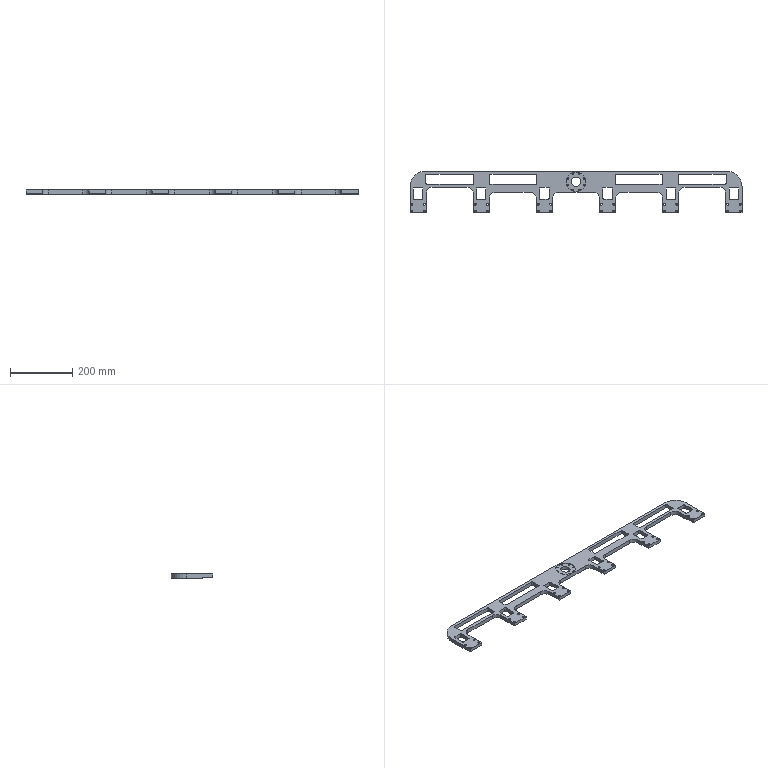NC program | NX | posted with a generic post | part box 1068 x 134 x 13 mm
Lines 5044 to 6064 of 9724:
(HOLE_MILLING_COPY , TOOL : D6)
N10038 T06 M6
N10040 G54
N10042 G17 G0 G90 X-25.869 Y43.715 S9500 M3
N10044 G43 Z30. H6
N10046 Z0.5
N10048 G94 G3 X-26.369 Y44.215 R0.5 F1400.
N10050 X-26.869 Y43.715 R0.5
N10052 X-26.869 Y43.715 Z0. I1. J0.
N10054 X-26.869 Y43.715 Z-0.5 I1. J0.
N10056 X-26.869 Y43.715 Z-1. I1. J0.
N10058 X-26.869 Y43.715 Z-1.5 I1. J0.
N10060 X-26.869 Y43.715 Z-2. I1. J0.
N10062 X-26.869 Y43.715 Z-2.5 I1. J0.
N10064 X-26.869 Y43.715 Z-3. I1. J0.
N10066 X-26.869 Y43.715 Z-3.5 I1. J0.
N10068 X-26.869 Y43.715 Z-4. I1. J0.
N10070 X-26.869 Y43.715 Z-4.5 I1. J0.
N10072 X-26.178 Y42.764 Z-4.6 R1.
N10074 X-24.918 Y43.406 R1.
N10076 X-26.178 Y42.764 R-1.
N10078 X-25.548 Y43.085 R0.5
N10080 X-25.869 Y43.715 R0.5
N10082 G0 Z30.
N10084 Y22.285
N10086 Z0.5
N10088 G3 X-26.369 Y22.785 R0.5
N10090 X-26.869 Y22.285 R0.5
N10092 X-26.869 Y22.285 Z0. I1. J0.
N10094 X-26.869 Y22.285 Z-0.5 I1. J0.
N10096 X-26.869 Y22.285 Z-1. I1. J0.
N10098 X-26.869 Y22.285 Z-1.5 I1. J0.
N10100 X-26.869 Y22.285 Z-2. I1. J0.
N10102 X-26.869 Y22.285 Z-2.5 I1. J0.
N10104 X-26.869 Y22.285 Z-3. I1. J0.
N10106 X-26.869 Y22.285 Z-3.5 I1. J0.
N10108 X-26.869 Y22.285 Z-4. I1. J0.
N10110 X-26.869 Y22.285 Z-4.5 I1. J0.
N10112 X-26.178 Y21.334 Z-4.6 R1.
N10114 X-24.918 Y21.976 R1.
N10116 X-26.178 Y21.334 R-1.
N10118 X-25.548 Y21.655 R0.5
N10120 X-25.869 Y22.285 R0.5
N10122 G0 Z30.
N10124 X-10.715 Y7.131
N10126 Z0.5
N10128 G3 X-11.215 Y7.631 R0.5
N10130 X-11.715 Y7.131 R0.5
N10132 X-11.715 Y7.131 Z0. I1. J0.
N10134 X-11.715 Y7.131 Z-0.5 I1. J0.
N10136 X-11.715 Y7.131 Z-1. I1. J0.
N10138 X-11.715 Y7.131 Z-1.5 I1. J0.
N10140 X-11.715 Y7.131 Z-2. I1. J0.
N10142 X-11.715 Y7.131 Z-2.5 I1. J0.
N10144 X-11.715 Y7.131 Z-3. I1. J0.
N10146 X-11.715 Y7.131 Z-3.5 I1. J0.
N10148 X-11.715 Y7.131 Z-4. I1. J0.
N10150 X-11.715 Y7.131 Z-4.5 I1. J0.
N10152 X-11.024 Y6.18 Z-4.6 R1.
N10154 X-9.764 Y6.822 R1.
N10156 X-11.024 Y6.18 R-1.
N10158 X-10.394 Y6.501 R0.5
N10160 X-10.715 Y7.131 R0.5
N10162 G0 Z30.
N10164 X10.715
N10166 Z0.5
N10168 G3 X10.215 Y7.631 R0.5
N10170 X9.715 Y7.131 R0.5
N10172 X9.715 Y7.131 Z0. I1. J0.
N10174 X9.715 Y7.131 Z-0.5 I1. J0.
N10176 X9.715 Y7.131 Z-1. I1. J0.
N10178 X9.715 Y7.131 Z-1.5 I1. J0.
N10180 X9.715 Y7.131 Z-2. I1. J0.
N10182 X9.715 Y7.131 Z-2.5 I1. J0.
N10184 X9.715 Y7.131 Z-3. I1. J0.
N10186 X9.715 Y7.131 Z-3.5 I1. J0.
N10188 X9.715 Y7.131 Z-4. I1. J0.
N10190 X9.715 Y7.131 Z-4.5 I1. J0.
N10192 X10.406 Y6.18 Z-4.6 R1.
N10194 X11.666 Y6.822 R1.
N10196 X10.406 Y6.18 R-1.
N10198 X11.036 Y6.501 R0.5
N10200 X10.715 Y7.131 R0.5
N10202 G0 Z30.
N10204 X25.869 Y22.285
N10206 Z0.5
N10208 G3 X25.369 Y22.785 R0.5
N10210 X24.869 Y22.285 R0.5
N10212 X24.869 Y22.285 Z0. I1. J0.
N10214 X24.869 Y22.285 Z-0.5 I1. J0.
N10216 X24.869 Y22.285 Z-1. I1. J0.
N10218 X24.869 Y22.285 Z-1.5 I1. J0.
N10220 X24.869 Y22.285 Z-2. I1. J0.
N10222 X24.869 Y22.285 Z-2.5 I1. J0.
N10224 X24.869 Y22.285 Z-3. I1. J0.
N10226 X24.869 Y22.285 Z-3.5 I1. J0.
N10228 X24.869 Y22.285 Z-4. I1. J0.
N10230 X24.869 Y22.285 Z-4.5 I1. J0.
N10232 X25.56 Y21.334 Z-4.6 R1.
N10234 X26.82 Y21.976 R1.
N10236 X25.56 Y21.334 R-1.
N10238 X26.19 Y21.655 R0.5
N10240 X25.869 Y22.285 R0.5
N10242 G0 Z30.
N10244 Y43.715
N10246 Z0.5
N10248 G3 X25.369 Y44.215 R0.5
N10250 X24.869 Y43.715 R0.5
N10252 X24.869 Y43.715 Z0. I1. J0.
N10254 X24.869 Y43.715 Z-0.5 I1. J0.
N10256 X24.869 Y43.715 Z-1. I1. J0.
N10258 X24.869 Y43.715 Z-1.5 I1. J0.
N10260 X24.869 Y43.715 Z-2. I1. J0.
N10262 X24.869 Y43.715 Z-2.5 I1. J0.
N10264 X24.869 Y43.715 Z-3. I1. J0.
N10266 X24.869 Y43.715 Z-3.5 I1. J0.
N10268 X24.869 Y43.715 Z-4. I1. J0.
N10270 X24.869 Y43.715 Z-4.5 I1. J0.
N10272 X25.56 Y42.764 Z-4.6 R1.
N10274 X26.82 Y43.406 R1.
N10276 X25.56 Y42.764 R-1.
N10278 X26.19 Y43.085 R0.5
N10280 X25.869 Y43.715 R0.5
N10282 G0 Z30.
N10284 X10.715 Y58.869
N10286 Z0.5
N10288 G3 X10.215 Y59.369 R0.5
N10290 X9.715 Y58.869 R0.5
N10292 X9.715 Y58.869 Z0. I1. J0.
N10294 X9.715 Y58.869 Z-0.5 I1. J0.
N10296 X9.715 Y58.869 Z-1. I1. J0.
N10298 X9.715 Y58.869 Z-1.5 I1. J0.
N10300 X9.715 Y58.869 Z-2. I1. J0.
N10302 X9.715 Y58.869 Z-2.5 I1. J0.
N10304 X9.715 Y58.869 Z-3. I1. J0.
N10306 X9.715 Y58.869 Z-3.5 I1. J0.
N10308 X9.715 Y58.869 Z-4. I1. J0.
N10310 X9.715 Y58.869 Z-4.5 I1. J0.
N10312 X10.406 Y57.918 Z-4.6 R1.
N10314 X11.666 Y58.56 R1.
N10316 X10.406 Y57.918 R-1.
N10318 X11.036 Y58.239 R0.5
N10320 X10.715 Y58.869 R0.5
N10322 G0 Z30.
N10324 X-10.715
N10326 Z0.5
N10328 G3 X-11.215 Y59.369 R0.5
N10330 X-11.715 Y58.869 R0.5
N10332 X-11.715 Y58.869 Z0. I1. J0.
N10334 X-11.715 Y58.869 Z-0.5 I1. J0.
N10336 X-11.715 Y58.869 Z-1. I1. J0.
N10338 X-11.715 Y58.869 Z-1.5 I1. J0.
N10340 X-11.715 Y58.869 Z-2. I1. J0.
N10342 X-11.715 Y58.869 Z-2.5 I1. J0.
N10344 X-11.715 Y58.869 Z-3. I1. J0.
N10346 X-11.715 Y58.869 Z-3.5 I1. J0.
N10348 X-11.715 Y58.869 Z-4. I1. J0.
N10350 X-11.715 Y58.869 Z-4.5 I1. J0.
N10352 X-11.024 Y57.918 Z-4.6 R1.
N10354 X-9.764 Y58.56 R1.
N10356 X-11.024 Y57.918 R-1.
N10358 X-10.394 Y58.239 R0.5
N10360 X-10.715 Y58.869 R0.5
N10362 G0 Z30.
(ZLEVEL_PROFILE_COPY_1_COPY , TOOL : D6)
N10364 X-131.879 Y29.2
N10366 Z-0.591
N10368 G1 Y28.003 F1000.
N10370 X-131.816 Y28.
N10372 X-129.6 F1650.
N10374 Y30.216
N10376 X-129.603 Y30.279
N10378 X-130.8
N10380 G0 X-131.879 Y29.2 Z-1.182
N10382 G1 Y28.003 F1000.
N10384 X-131.816 Y28.
N10386 X-129.6 F1650.
N10388 Y30.216
N10390 X-129.603 Y30.279
N10392 X-130.8
N10394 G0 X-131.879 Y29.2 Z-1.773
N10396 G1 Y28.003 F1000.
N10398 X-131.816 Y28.
N10400 X-129.6 F1650.
N10402 Y30.216
N10404 X-129.603 Y30.279
N10406 X-130.8
N10408 G0 X-131.879 Y29.2 Z-2.364
N10410 G1 Y28.003 F1000.
N10412 X-131.816 Y28.
N10414 X-129.6 F1650.
N10416 Y30.216
N10418 X-129.603 Y30.279
N10420 X-130.8
N10422 G0 X-131.879 Y29.2 Z-2.955
N10424 G1 Y28.003 F1000.
N10426 X-131.816 Y28.
N10428 X-129.6 F1650.
N10430 Y30.216
N10432 X-129.603 Y30.279
N10434 X-130.8
N10436 G0 X-131.879 Y29.2 Z-3.545
N10438 G1 Y28.003 F1000.
N10440 X-131.816 Y28.
N10442 X-129.6 F1650.
N10444 Y30.216
N10446 X-129.603 Y30.279
N10448 X-130.8
N10450 G0 X-131.879 Y29.2 Z-4.136
N10452 G1 Y28.003 F1000.
N10454 X-131.816 Y28.
N10456 X-129.6 F1650.
N10458 Y30.216
N10460 X-129.603 Y30.279
N10462 X-130.8
N10464 G0 X-131.879 Y29.2 Z-4.727
N10466 G1 Y28.003 F1000.
N10468 X-131.816 Y28.
N10470 X-129.6 F1650.
N10472 Y30.216
N10474 X-129.603 Y30.279
N10476 X-130.8
N10478 G0 X-131.879 Y29.2 Z-5.318
N10480 G1 Y28.003 F1000.
N10482 X-131.816 Y28.
N10484 X-129.6 F1650.
N10486 Y30.216
N10488 X-129.603 Y30.279
N10490 X-130.8
N10492 G0 X-131.879 Y29.2 Z-5.909
N10494 G1 Y28.003 F1000.
N10496 X-131.816 Y28.
N10498 X-129.6 F1650.
N10500 Y30.216
N10502 X-129.603 Y30.279
N10504 X-130.8
N10506 G0 X-131.879 Y29.2 Z-6.5
N10508 G1 Y28.003 F1000.
N10510 X-131.816 Y28.
N10512 X-129.6 F1650.
N10514 Y30.216
N10516 X-129.603 Y30.279
N10518 X-130.8
N10520 G0 X-131.879 Y29.2 Z-7.091
N10522 G1 Y28.003 F1000.
N10524 X-131.816 Y28.
N10526 X-129.6 F1650.
N10528 Y30.216
N10530 X-129.603 Y30.279
N10532 X-130.8
N10534 G0 X-131.879 Y29.2 Z-7.682
N10536 G1 Y28.003 F1000.
N10538 X-131.816 Y28.
N10540 X-129.6 F1650.
N10542 Y30.216
N10544 X-129.603 Y30.279
N10546 X-130.8
N10548 G0 X-131.893 Y29.2 Z-8.273
N10550 G1 Y28.003 F1000.
N10552 X-131.83 Y28.
N10554 X-129.6 F1650.
N10556 Y30.218
N10558 X-129.603 Y30.281
N10560 X-130.8
N10562 G0 X-131.893 Y29.2 Z-8.864
N10564 G1 Y28.003 F1000.
N10566 X-131.83 Y28.
N10568 X-129.6 F1650.
N10570 Y30.218
N10572 X-129.603 Y30.281
N10574 X-130.8
N10576 G0 X-131.893 Y29.2 Z-9.455
N10578 G1 Y28.003 F1000.
N10580 X-131.83 Y28.
N10582 X-129.6 F1650.
N10584 Y30.218
N10586 X-129.603 Y30.281
N10588 X-130.8
N10590 G0 X-131.893 Y29.2 Z-10.045
N10592 G1 Y28.003 F1000.
N10594 X-131.83 Y28.
N10596 X-129.6 F1650.
N10598 Y30.218
N10600 X-129.603 Y30.281
N10602 X-130.8
N10604 G0 X-131.893 Y29.2 Z-10.636
N10606 G1 Y28.003 F1000.
N10608 X-131.83 Y28.
N10610 X-129.6 F1650.
N10612 Y30.218
N10614 X-129.603 Y30.281
N10616 X-130.8
N10618 G0 X-131.893 Y29.2 Z-11.227
N10620 G1 Y28.003 F1000.
N10622 X-131.83 Y28.
N10624 X-129.6 F1650.
N10626 Y30.218
N10628 X-129.603 Y30.281
N10630 X-130.8
N10632 G0 X-131.893 Y29.2 Z-11.818
N10634 G1 Y28.003 F1000.
N10636 X-131.83 Y28.
N10638 X-129.6 F1650.
N10640 Y30.218
N10642 X-129.603 Y30.281
N10644 X-130.8
N10646 G0 X-131.893 Y29.2 Z-12.409
N10648 G1 Y28.003 F1000.
N10650 X-131.83 Y28.
N10652 X-129.6 F1650.
N10654 Y30.218
N10656 X-129.603 Y30.281
N10658 X-130.8
N10660 G0 X-131.893 Y29.2 Z-13.
N10662 G1 Y28.003 F1000.
N10664 X-131.83 Y28.
N10666 X-129.6 F1650.
N10668 Y30.218
N10670 X-129.603 Y30.281
N10672 X-130.8
N10674 G0 Z30.
N10676 Y51.721
N10678 Z-0.591
N10680 G1 X-129.603 F1000.
N10682 X-129.6 Y51.784
N10684 Y54. F1650.
N10686 X-131.816
N10688 X-131.879 Y53.997
N10690 Y52.8
N10692 G0 X-130.8 Y51.721 Z-1.182
N10694 G1 X-129.603 F1000.
N10696 X-129.6 Y51.784
N10698 Y54. F1650.
N10700 X-131.816
N10702 X-131.879 Y53.997
N10704 Y52.8
N10706 G0 X-130.8 Y51.721 Z-1.773
N10708 G1 X-129.603 F1000.
N10710 X-129.6 Y51.784
N10712 Y54. F1650.
N10714 X-131.816
N10716 X-131.879 Y53.997
N10718 Y52.8
N10720 G0 X-130.8 Y51.721 Z-2.364
N10722 G1 X-129.603 F1000.
N10724 X-129.6 Y51.784
N10726 Y54. F1650.
N10728 X-131.816
N10730 X-131.879 Y53.997
N10732 Y52.8
N10734 G0 X-130.8 Y51.721 Z-2.955
N10736 G1 X-129.603 F1000.
N10738 X-129.6 Y51.784
N10740 Y54. F1650.
N10742 X-131.816
N10744 X-131.879 Y53.997
N10746 Y52.8
N10748 G0 X-130.8 Y51.721 Z-3.545
N10750 G1 X-129.603 F1000.
N10752 X-129.6 Y51.784
N10754 Y54. F1650.
N10756 X-131.816
N10758 X-131.879 Y53.997
N10760 Y52.8
N10762 G0 X-130.8 Y51.721 Z-4.136
N10764 G1 X-129.603 F1000.
N10766 X-129.6 Y51.784
N10768 Y54. F1650.
N10770 X-131.816
N10772 X-131.879 Y53.997
N10774 Y52.8
N10776 G0 X-130.8 Y51.721 Z-4.727
N10778 G1 X-129.603 F1000.
N10780 X-129.6 Y51.784
N10782 Y54. F1650.
N10784 X-131.816
N10786 X-131.879 Y53.997
N10788 Y52.8
N10790 G0 X-130.8 Y51.721 Z-5.318
N10792 G1 X-129.603 F1000.
N10794 X-129.6 Y51.784
N10796 Y54. F1650.
N10798 X-131.816
N10800 X-131.879 Y53.997
N10802 Y52.8
N10804 G0 X-130.8 Y51.721 Z-5.909
N10806 G1 X-129.603 F1000.
N10808 X-129.6 Y51.784
N10810 Y54. F1650.
N10812 X-131.816
N10814 X-131.879 Y53.997
N10816 Y52.8
N10818 G0 X-130.8 Y51.721 Z-6.5
N10820 G1 X-129.603 F1000.
N10822 X-129.6 Y51.784
N10824 Y54. F1650.
N10826 X-131.816
N10828 X-131.879 Y53.997
N10830 Y52.8
N10832 G0 X-130.8 Y51.721 Z-7.091
N10834 G1 X-129.603 F1000.
N10836 X-129.6 Y51.784
N10838 Y54. F1650.
N10840 X-131.816
N10842 X-131.879 Y53.997
N10844 Y52.8
N10846 G0 X-130.8 Y51.721 Z-7.682
N10848 G1 X-129.603 F1000.
N10850 X-129.6 Y51.784
N10852 Y54. F1650.
N10854 X-131.816
N10856 X-131.879 Y53.997
N10858 Y52.8
N10860 G0 X-130.8 Y51.726 Z-8.273
N10862 G1 X-129.603 F1000.
N10864 X-129.6 Y51.789
N10866 Y53.988 F1650.
N10868 Y54.
N10870 X-131.81
N10872 X-131.873 Y53.997
N10874 Y52.8
N10876 G0 X-130.8 Y51.726 Z-8.864
N10878 G1 X-129.603 F1000.
N10880 X-129.6 Y51.789
N10882 Y53.988 F1650.
N10884 Y54.
N10886 X-131.81
N10888 X-131.873 Y53.997
N10890 Y52.8
N10892 G0 X-130.8 Y51.726 Z-9.455
N10894 G1 X-129.603 F1000.
N10896 X-129.6 Y51.789
N10898 Y53.988 F1650.
N10900 Y54.
N10902 X-131.81
N10904 X-131.873 Y53.997
N10906 Y52.8
N10908 G0 X-130.8 Y51.726 Z-10.045
N10910 G1 X-129.603 F1000.
N10912 X-129.6 Y51.789
N10914 Y53.988 F1650.
N10916 Y54.
N10918 X-131.81
N10920 X-131.873 Y53.997
N10922 Y52.8
N10924 G0 X-130.8 Y51.726 Z-10.636
N10926 G1 X-129.603 F1000.
N10928 X-129.6 Y51.789
N10930 Y53.988 F1650.
N10932 Y54.
N10934 X-131.81
N10936 X-131.873 Y53.997
N10938 Y52.8
N10940 G0 X-130.8 Y51.726 Z-11.227
N10942 G1 X-129.603 F1000.
N10944 X-129.6 Y51.789
N10946 Y53.988 F1650.
N10948 Y54.
N10950 X-131.81
N10952 X-131.873 Y53.997
N10954 Y52.8
N10956 G0 X-130.8 Y51.726 Z-11.818
N10958 G1 X-129.603 F1000.
N10960 X-129.6 Y51.789
N10962 Y53.988 F1650.
N10964 Y54.
N10966 X-131.81
N10968 X-131.873 Y53.997
N10970 Y52.8
N10972 G0 X-130.8 Y51.726 Z-12.409
N10974 G1 X-129.603 F1000.
N10976 X-129.6 Y51.789
N10978 Y53.988 F1650.
N10980 Y54.
N10982 X-131.81
N10984 X-131.873 Y53.997
N10986 Y52.8
N10988 G0 X-130.8 Y51.726 Z-13.
N10990 G1 X-129.603 F1000.
N10992 X-129.6 Y51.789
N10994 Y53.988 F1650.
N10996 Y54.
N10998 X-131.81
N11000 X-131.873 Y53.997
N11002 Y52.8
N11004 G0 Z30.
N11006 X-274.521
N11008 Z-0.591
N11010 G1 Y53.997 F1000.
N11012 X-274.584 Y54.
N11014 X-276.8 F1650.
N11016 Y51.784
N11018 X-276.797 Y51.721
N11020 X-275.6
N11022 G0 X-274.521 Y52.8 Z-1.182
N11024 G1 Y53.997 F1000.
N11026 X-274.584 Y54.
N11028 X-276.8 F1650.
N11030 Y51.784
N11032 X-276.797 Y51.721
N11034 X-275.6
N11036 G0 X-274.521 Y52.8 Z-1.773
N11038 G1 Y53.997 F1000.
N11040 X-274.584 Y54.
N11042 X-276.8 F1650.
N11044 Y51.784
N11046 X-276.797 Y51.721
N11048 X-275.6
N11050 G0 X-274.521 Y52.8 Z-2.364
N11052 G1 Y53.997 F1000.
N11054 X-274.584 Y54.
N11056 X-276.8 F1650.
N11058 Y51.784
N11060 X-276.797 Y51.721
N11062 X-275.6
N11064 G0 X-274.521 Y52.8 Z-2.955
N11066 G1 Y53.997 F1000.
N11068 X-274.584 Y54.
N11070 X-276.8 F1650.
N11072 Y51.784
N11074 X-276.797 Y51.721
N11076 X-275.6
N11078 G0 X-274.521 Y52.8 Z-3.545
N11080 G1 Y53.997 F1000.
N11082 X-274.584 Y54.
N11084 X-276.8 F1650.
N11086 Y51.784
N11088 X-276.797 Y51.721
N11090 X-275.6
N11092 G0 X-274.521 Y52.8 Z-4.136
N11094 G1 Y53.997 F1000.
N11096 X-274.584 Y54.
N11098 X-276.8 F1650.
N11100 Y51.784
N11102 X-276.797 Y51.721
N11104 X-275.6
N11106 G0 X-274.521 Y52.8 Z-4.727
N11108 G1 Y53.997 F1000.
N11110 X-274.584 Y54.
N11112 X-276.8 F1650.
N11114 Y51.784
N11116 X-276.797 Y51.721
N11118 X-275.6
N11120 G0 X-274.521 Y52.8 Z-5.318
N11122 G1 Y53.997 F1000.
N11124 X-274.584 Y54.
N11126 X-276.8 F1650.
N11128 Y51.784
N11130 X-276.797 Y51.721
N11132 X-275.6
N11134 G0 X-274.521 Y52.8 Z-5.909
N11136 G1 Y53.997 F1000.
N11138 X-274.584 Y54.
N11140 X-276.8 F1650.
N11142 Y51.784
N11144 X-276.797 Y51.721
N11146 X-275.6
N11148 G0 X-274.521 Y52.8 Z-6.5
N11150 G1 Y53.997 F1000.
N11152 X-274.584 Y54.
N11154 X-276.8 F1650.
N11156 Y51.784
N11158 X-276.797 Y51.721
N11160 X-275.6
N11162 G0 X-274.521 Y52.8 Z-7.091
N11164 G1 Y53.997 F1000.
N11166 X-274.584 Y54.
N11168 X-276.8 F1650.
N11170 Y51.784
N11172 X-276.797 Y51.721
N11174 X-275.6
N11176 G0 X-274.521 Y52.8 Z-7.682
N11178 G1 Y53.997 F1000.
N11180 X-274.584 Y54.
N11182 X-276.8 F1650.
N11184 Y51.784
N11186 X-276.797 Y51.721
N11188 X-275.6
N11190 G0 X-274.534 Y52.8 Z-8.273
N11192 G1 Y53.997 F1000.
N11194 X-274.597 Y54.
N11196 X-276.8 F1650.
N11198 Y51.785
N11200 X-276.797 Y51.723
N11202 X-275.6
N11204 G0 X-274.534 Y52.8 Z-8.864
N11206 G1 Y53.997 F1000.
N11208 X-274.597 Y54.
N11210 X-276.8 F1650.
N11212 Y51.785
N11214 X-276.797 Y51.723
N11216 X-275.6
N11218 G0 X-274.534 Y52.8 Z-9.455
N11220 G1 Y53.997 F1000.
N11222 X-274.597 Y54.
N11224 X-276.8 F1650.
N11226 Y51.785
N11228 X-276.797 Y51.723
N11230 X-275.6
N11232 G0 X-274.534 Y52.8 Z-10.045
N11234 G1 Y53.997 F1000.
N11236 X-274.597 Y54.
N11238 X-276.8 F1650.
N11240 Y51.785
N11242 X-276.797 Y51.723
N11244 X-275.6
N11246 G0 X-274.534 Y52.8 Z-10.636
N11248 G1 Y53.997 F1000.
N11250 X-274.597 Y54.
N11252 X-276.8 F1650.
N11254 Y51.785
N11256 X-276.797 Y51.723
N11258 X-275.6
N11260 G0 X-274.534 Y52.8 Z-11.227
N11262 G1 Y53.997 F1000.
N11264 X-274.597 Y54.
N11266 X-276.8 F1650.
N11268 Y51.785
N11270 X-276.797 Y51.723
N11272 X-275.6
N11274 G0 X-274.534 Y52.8 Z-11.818
N11276 G1 Y53.997 F1000.
N11278 X-274.597 Y54.
N11280 X-276.8 F1650.
N11282 Y51.785
N11284 X-276.797 Y51.723
N11286 X-275.6
N11288 G0 X-274.534 Y52.8 Z-12.409
N11290 G1 Y53.997 F1000.
N11292 X-274.597 Y54.
N11294 X-276.8 F1650.
N11296 Y51.785
N11298 X-276.797 Y51.723
N11300 X-275.6
N11302 G0 X-274.534 Y52.8 Z-13.
N11304 G1 Y53.997 F1000.
N11306 X-274.597 Y54.
N11308 X-276.8 F1650.
N11310 Y51.785
N11312 X-276.797 Y51.723
N11314 X-275.6
N11316 G0 Z30.
N11318 Y30.279
N11320 Z-0.591
N11322 G1 X-276.797 F1000.
N11324 X-276.8 Y30.216
N11326 Y28. F1650.
N11328 X-274.584
N11330 X-274.521 Y28.003
N11332 Y29.2
N11334 G0 X-275.6 Y30.279 Z-1.182
N11336 G1 X-276.797 F1000.
N11338 X-276.8 Y30.216
N11340 Y28. F1650.
N11342 X-274.584
N11344 X-274.521 Y28.003
N11346 Y29.2
N11348 G0 X-275.6 Y30.279 Z-1.773
N11350 G1 X-276.797 F1000.
N11352 X-276.8 Y30.216
N11354 Y28. F1650.
N11356 X-274.584
N11358 X-274.521 Y28.003
N11360 Y29.2
N11362 G0 X-275.6 Y30.279 Z-2.364
N11364 G1 X-276.797 F1000.
N11366 X-276.8 Y30.216
N11368 Y28. F1650.
N11370 X-274.584
N11372 X-274.521 Y28.003
N11374 Y29.2
N11376 G0 X-275.6 Y30.279 Z-2.955
N11378 G1 X-276.797 F1000.
N11380 X-276.8 Y30.216
N11382 Y28. F1650.
N11384 X-274.584
N11386 X-274.521 Y28.003
N11388 Y29.2
N11390 G0 X-275.6 Y30.279 Z-3.545
N11392 G1 X-276.797 F1000.
N11394 X-276.8 Y30.216
N11396 Y28. F1650.
N11398 X-274.584
N11400 X-274.521 Y28.003
N11402 Y29.2
N11404 G0 X-275.6 Y30.279 Z-4.136
N11406 G1 X-276.797 F1000.
N11408 X-276.8 Y30.216
N11410 Y28. F1650.
N11412 X-274.584
N11414 X-274.521 Y28.003
N11416 Y29.2
N11418 G0 X-275.6 Y30.279 Z-4.727
N11420 G1 X-276.797 F1000.
N11422 X-276.8 Y30.216
N11424 Y28. F1650.
N11426 X-274.584
N11428 X-274.521 Y28.003
N11430 Y29.2
N11432 G0 X-275.6 Y30.279 Z-5.318
N11434 G1 X-276.797 F1000.
N11436 X-276.8 Y30.216
N11438 Y28. F1650.
N11440 X-274.584
N11442 X-274.521 Y28.003
N11444 Y29.2
N11446 G0 X-275.6 Y30.279 Z-5.909
N11448 G1 X-276.797 F1000.
N11450 X-276.8 Y30.216
N11452 Y28. F1650.
N11454 X-274.584
N11456 X-274.521 Y28.003
N11458 Y29.2
N11460 G0 X-275.6 Y30.279 Z-6.5
N11462 G1 X-276.797 F1000.
N11464 X-276.8 Y30.216
N11466 Y28. F1650.
N11468 X-274.584
N11470 X-274.521 Y28.003
N11472 Y29.2
N11474 G0 X-275.6 Y30.279 Z-7.091
N11476 G1 X-276.797 F1000.
N11478 X-276.8 Y30.216
N11480 Y28. F1650.
N11482 X-274.584
N11484 X-274.521 Y28.003
N11486 Y29.2
N11488 G0 X-275.6 Y30.279 Z-7.682
N11490 G1 X-276.797 F1000.
N11492 X-276.8 Y30.216
N11494 Y28. F1650.
N11496 X-274.584
N11498 X-274.521 Y28.003
N11500 Y29.2
N11502 G0 X-275.6 Y30.278 Z-8.273
N11504 G1 X-276.797 F1000.
N11506 X-276.8 Y30.216
N11508 Y28. F1650.
N11510 X-274.584
N11512 X-274.521 Y28.003
N11514 Y29.2
N11516 G0 X-275.6 Y30.278 Z-8.864
N11518 G1 X-276.797 F1000.
N11520 X-276.8 Y30.216
N11522 Y28. F1650.
N11524 X-274.584
N11526 X-274.521 Y28.003
N11528 Y29.2
N11530 G0 X-275.6 Y30.278 Z-9.455
N11532 G1 X-276.797 F1000.
N11534 X-276.8 Y30.216
N11536 Y28. F1650.
N11538 X-274.584
N11540 X-274.521 Y28.003
N11542 Y29.2
N11544 G0 X-275.6 Y30.278 Z-10.045
N11546 G1 X-276.797 F1000.
N11548 X-276.8 Y30.216
N11550 Y28. F1650.
N11552 X-274.584
N11554 X-274.521 Y28.003
N11556 Y29.2
N11558 G0 X-275.6 Y30.278 Z-10.636
N11560 G1 X-276.797 F1000.
N11562 X-276.8 Y30.216
N11564 Y28. F1650.
N11566 X-274.584
N11568 X-274.521 Y28.003
N11570 Y29.2
N11572 G0 X-275.6 Y30.278 Z-11.227
N11574 G1 X-276.797 F1000.
N11576 X-276.8 Y30.216
N11578 Y28. F1650.
N11580 X-274.584
N11582 X-274.521 Y28.003
N11584 Y29.2
N11586 G0 X-275.6 Y30.278 Z-11.818
N11588 G1 X-276.797 F1000.
N11590 X-276.8 Y30.216
N11592 Y28. F1650.
N11594 X-274.584
N11596 X-274.521 Y28.003
N11598 Y29.2
N11600 G0 X-275.6 Y30.278 Z-12.409
N11602 G1 X-276.797 F1000.
N11604 X-276.8 Y30.216
N11606 Y28. F1650.
N11608 X-274.584
N11610 X-274.521 Y28.003
N11612 Y29.2
N11614 G0 X-275.6 Y30.278 Z-13.
N11616 G1 X-276.797 F1000.
N11618 X-276.8 Y30.216
N11620 Y28. F1650.
N11622 X-274.584
N11624 X-274.521 Y28.003
N11626 Y29.2
N11628 G0 Z30.
N11630 X-335.079
N11632 Z-0.591
N11634 G1 Y28.003 F1000.
N11636 X-335.016 Y28.
N11638 X-332.8 F1650.
N11640 Y30.216
N11642 X-332.803 Y30.279
N11644 X-334.
N11646 G0 X-335.079 Y29.2 Z-1.182
N11648 G1 Y28.003 F1000.
N11650 X-335.016 Y28.
N11652 X-332.8 F1650.
N11654 Y30.216
N11656 X-332.803 Y30.279
N11658 X-334.
N11660 G0 X-335.079 Y29.2 Z-1.773
N11662 G1 Y28.003 F1000.
N11664 X-335.016 Y28.
N11666 X-332.8 F1650.
N11668 Y30.216
N11670 X-332.803 Y30.279
N11672 X-334.
N11674 G0 X-335.079 Y29.2 Z-2.364
N11676 G1 Y28.003 F1000.
N11678 X-335.016 Y28.
N11680 X-332.8 F1650.
N11682 Y30.216
N11684 X-332.803 Y30.279
N11686 X-334.
N11688 G0 X-335.079 Y29.2 Z-2.955
N11690 G1 Y28.003 F1000.
N11692 X-335.016 Y28.
N11694 X-332.8 F1650.
N11696 Y30.216
N11698 X-332.803 Y30.279
N11700 X-334.
N11702 G0 X-335.079 Y29.2 Z-3.545
N11704 G1 Y28.003 F1000.
N11706 X-335.016 Y28.
N11708 X-332.8 F1650.
N11710 Y30.216
N11712 X-332.803 Y30.279
N11714 X-334.
N11716 G0 X-335.079 Y29.2 Z-4.136
N11718 G1 Y28.003 F1000.
N11720 X-335.016 Y28.
N11722 X-332.8 F1650.
N11724 Y30.216
N11726 X-332.803 Y30.279
N11728 X-334.
N11730 G0 X-335.079 Y29.2 Z-4.727
N11732 G1 Y28.003 F1000.
N11734 X-335.016 Y28.
N11736 X-332.8 F1650.
N11738 Y30.216
N11740 X-332.803 Y30.279
N11742 X-334.
N11744 G0 X-335.079 Y29.2 Z-5.318
N11746 G1 Y28.003 F1000.
N11748 X-335.016 Y28.
N11750 X-332.8 F1650.
N11752 Y30.216
N11754 X-332.803 Y30.279
N11756 X-334.
N11758 G0 X-335.079 Y29.2 Z-5.909
N11760 G1 Y28.003 F1000.
N11762 X-335.016 Y28.
N11764 X-332.8 F1650.
N11766 Y30.216
N11768 X-332.803 Y30.279
N11770 X-334.
N11772 G0 X-335.079 Y29.2 Z-6.5
N11774 G1 Y28.003 F1000.
N11776 X-335.016 Y28.
N11778 X-332.8 F1650.
N11780 Y30.216
N11782 X-332.803 Y30.279
N11784 X-334.
N11786 G0 X-335.079 Y29.2 Z-7.091
N11788 G1 Y28.003 F1000.
N11790 X-335.016 Y28.
N11792 X-332.8 F1650.
N11794 Y30.216
N11796 X-332.803 Y30.279
N11798 X-334.
N11800 G0 X-335.079 Y29.2 Z-7.682
N11802 G1 Y28.003 F1000.
N11804 X-335.016 Y28.
N11806 X-332.8 F1650.
N11808 Y30.216
N11810 X-332.803 Y30.279
N11812 X-334.
N11814 G0 X-335.089 Y29.2 Z-8.273
N11816 G1 Y28.003 F1000.
N11818 X-335.026 Y28.
N11820 X-332.8 F1650.
N11822 Y30.218
N11824 X-332.803 Y30.281
N11826 X-334.
N11828 G0 X-335.089 Y29.2 Z-8.864
N11830 G1 Y28.003 F1000.
N11832 X-335.026 Y28.
N11834 X-332.8 F1650.
N11836 Y30.218
N11838 X-332.803 Y30.281
N11840 X-334.
N11842 G0 X-335.089 Y29.2 Z-9.455
N11844 G1 Y28.003 F1000.
N11846 X-335.026 Y28.
N11848 X-332.8 F1650.
N11850 Y30.218
N11852 X-332.803 Y30.281
N11854 X-334.
N11856 G0 X-335.089 Y29.2 Z-10.045
N11858 G1 Y28.003 F1000.
N11860 X-335.026 Y28.
N11862 X-332.8 F1650.
N11864 Y30.218
N11866 X-332.803 Y30.281
N11868 X-334.
N11870 G0 X-335.089 Y29.2 Z-10.636
N11872 G1 Y28.003 F1000.
N11874 X-335.026 Y28.
N11876 X-332.8 F1650.
N11878 Y30.218
N11880 X-332.803 Y30.281
N11882 X-334.
N11884 G0 X-335.089 Y29.2 Z-11.227
N11886 G1 Y28.003 F1000.
N11888 X-335.026 Y28.
N11890 X-332.8 F1650.
N11892 Y30.218
N11894 X-332.803 Y30.281
N11896 X-334.
N11898 G0 X-335.089 Y29.2 Z-11.818
N11900 G1 Y28.003 F1000.
N11902 X-335.026 Y28.
N11904 X-332.8 F1650.
N11906 Y30.218
N11908 X-332.803 Y30.281
N11910 X-334.
N11912 G0 X-335.089 Y29.2 Z-12.409
N11914 G1 Y28.003 F1000.
N11916 X-335.026 Y28.
N11918 X-332.8 F1650.
N11920 Y30.218
N11922 X-332.803 Y30.281
N11924 X-334.
N11926 G0 X-335.089 Y29.2 Z-13.
N11928 G1 Y28.003 F1000.
N11930 X-335.026 Y28.
N11932 X-332.8 F1650.
N11934 Y30.218
N11936 X-332.803 Y30.281
N11938 X-334.
N11940 G0 Z30.
N11942 Y51.721
N11944 Z-0.591
N11946 G1 X-332.803 F1000.
N11948 X-332.8 Y51.784
N11950 Y54. F1650.
N11952 X-335.016
N11954 X-335.079 Y53.997
N11956 Y52.8
N11958 G0 X-334. Y51.721 Z-1.182
N11960 G1 X-332.803 F1000.
N11962 X-332.8 Y51.784
N11964 Y54. F1650.
N11966 X-335.016
N11968 X-335.079 Y53.997
N11970 Y52.8
N11972 G0 X-334. Y51.721 Z-1.773
N11974 G1 X-332.803 F1000.
N11976 X-332.8 Y51.784
N11978 Y54. F1650.
N11980 X-335.016
N11982 X-335.079 Y53.997
N11984 Y52.8
N11986 G0 X-334. Y51.721 Z-2.364
N11988 G1 X-332.803 F1000.
N11990 X-332.8 Y51.784
N11992 Y54. F1650.
N11994 X-335.016
N11996 X-335.079 Y53.997
N11998 Y52.8
N12000 G0 X-334. Y51.721 Z-2.955
N12002 G1 X-332.803 F1000.
N12004 X-332.8 Y51.784
N12006 Y54. F1650.
N12008 X-335.016
N12010 X-335.079 Y53.997
N12012 Y52.8
N12014 G0 X-334. Y51.721 Z-3.545
N12016 G1 X-332.803 F1000.
N12018 X-332.8 Y51.784
N12020 Y54. F1650.
N12022 X-335.016
N12024 X-335.079 Y53.997
N12026 Y52.8
N12028 G0 X-334. Y51.721 Z-4.136
N12030 G1 X-332.803 F1000.
N12032 X-332.8 Y51.784
N12034 Y54. F1650.
N12036 X-335.016
N12038 X-335.079 Y53.997
N12040 Y52.8
N12042 G0 X-334. Y51.721 Z-4.727
N12044 G1 X-332.803 F1000.
N12046 X-332.8 Y51.784
N12048 Y54. F1650.
N12050 X-335.016
N12052 X-335.079 Y53.997
N12054 Y52.8
N12056 G0 X-334. Y51.721 Z-5.318
N12058 G1 X-332.803 F1000.
N12060 X-332.8 Y51.784
N12062 Y54. F1650.
N12064 X-335.016
N12066 X-335.079 Y53.997